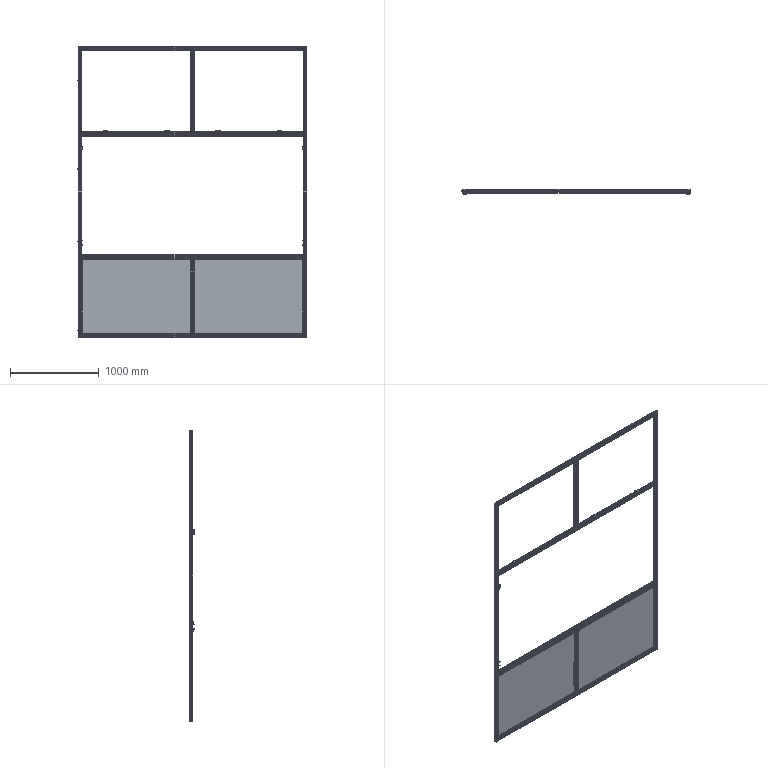Part | SolidWorks | features ReferencePattern 57, LocalLPattern 9, CompositeCurve 4, DerivedHolePattern 2 | 141 solids | 4787 faces | volume 23168671 mm3 | plane 3014 | cylinder 1241 | cone 516 | spline 16 | commonest cylinder face diameters 6.8 x172 2 x116 8 x96 4 x76 19 x72 6 x58